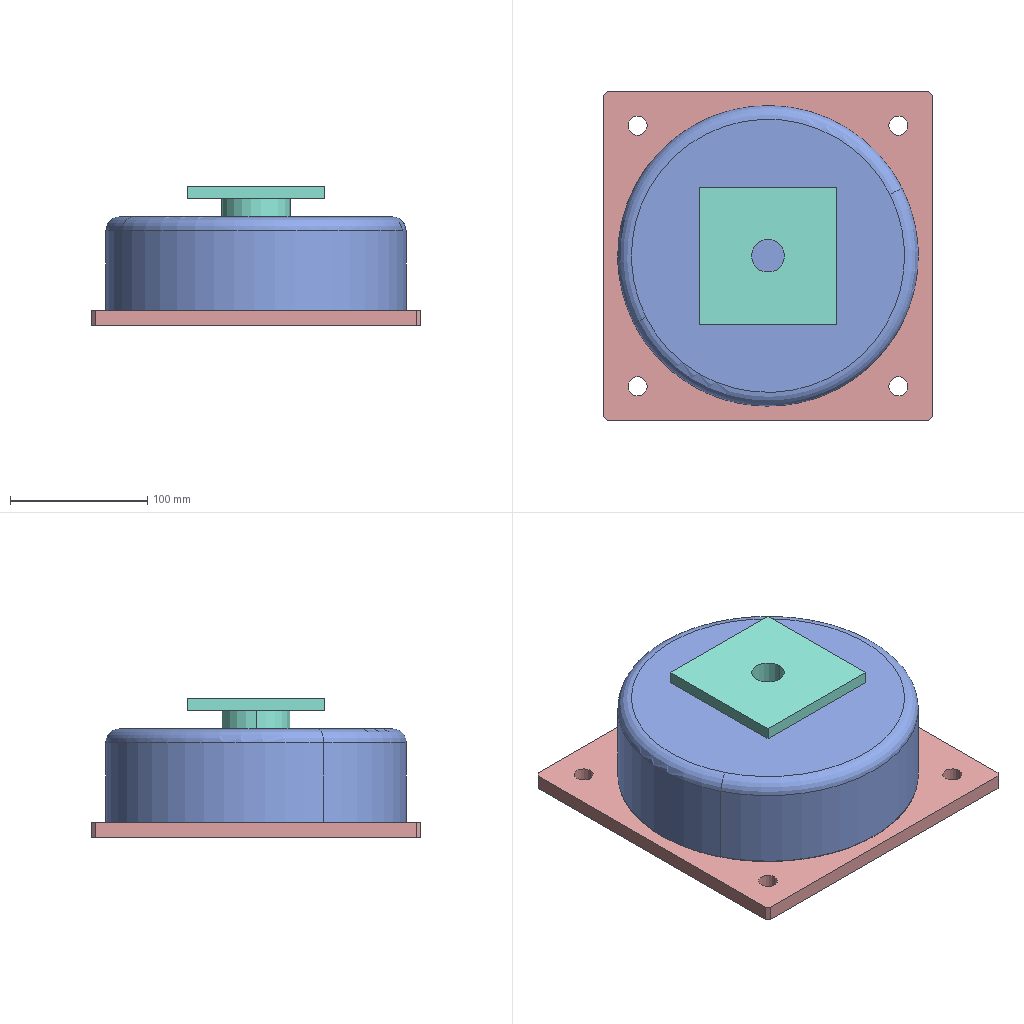Assembly | SolidWorks | 6 different items | 6 placed | box 240 x 240 x 102 mm
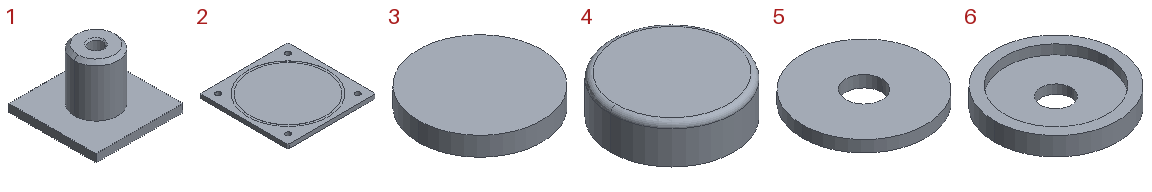Parts list (item | quantity | size | volume | features):
1 | x1 | 100 x 100 x 68 mm | 174571 mm3 | features Chamfer 1, Extrusion 1, HoleWzd 1, ICE 1
2 | x1 | 240 x 240 x 11 mm | 624621 mm3 | features ICE 2, Chamfer 1, Extrusion 1
3 | x1 | 149 x 149 x 23 mm | 401042 mm3 | features Extrusion 1
4 | x1 | 219 x 219 x 69 mm | 466703 mm3 | features Fillet 2, Extrusion 1, Shell 1
5 | x1 | 169.5 x 169.5 x 16 mm | 329619 mm3 | features Extrusion 1
6 | x1 | 206 x 206 x 31 mm | 639393 mm3 | features Extrusion 1, ICE 1
Mates (type | each side: item.copy, entity, surface, feature):
Concentric | 2.1 edge | 4.1 edge
Coincident | 2.1 face plane Cut-Extrude1 | 4.1 face plane Boss-Extrude1
Concentric | 2.1 edge | 3.1 face cylinder Boss-Extrude1
Coincident | 2.1 face plane Boss-Extrude1 | 3.1 face plane Boss-Extrude1
Concentric | 3.1 face cylinder Boss-Extrude1 | 5.1 face cylinder Boss-Extrude1
Coincident | 3.1 face plane Boss-Extrude1 | 5.1 face plane Boss-Extrude1
Parallel | 2.1 face plane Boss-Extrude1 | 1.1 face plane Boss-Extrude1
Coincident | 3.1 face plane Boss-Extrude1 | 1.1 face plane Boss-Extrude2
Concentric | 5.1 face cylinder Boss-Extrude1 | 6.1 face cylinder Boss-Extrude1
Coincident | 5.1 face plane Boss-Extrude1 | 6.1 face plane Boss-Extrude2